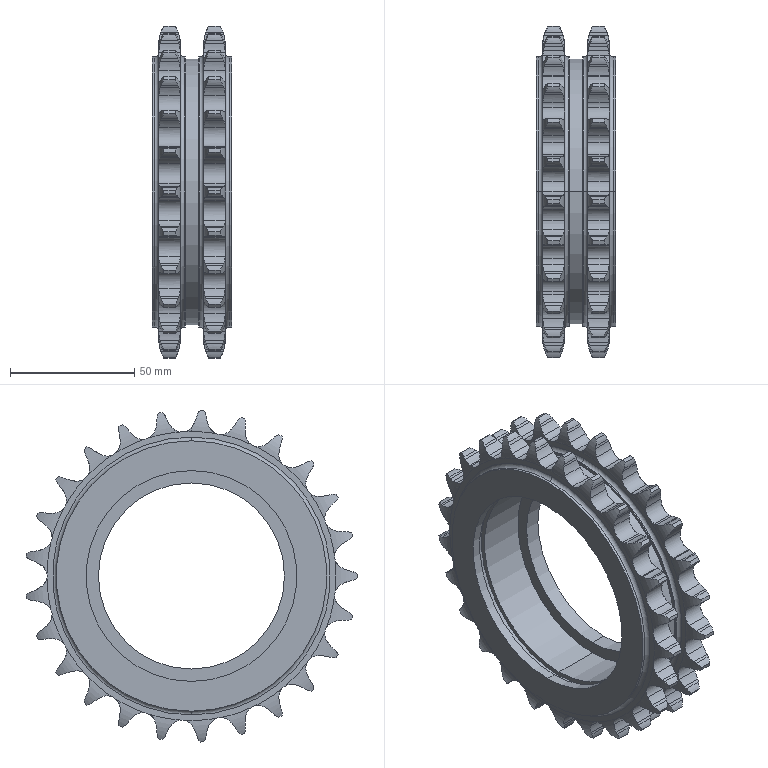Part | SolidWorks | features BaseBody 1 | 1 solid | 563 faces | box 32.003 x 133.563 x 133.823 mm | volume 164866 mm3 | cylinder 340 | torus 112 | plane 111 | commonest cylinder face diameters 14.66 x104 26.567 x104 10.311 x64 134 x50 109 x8 85 x4